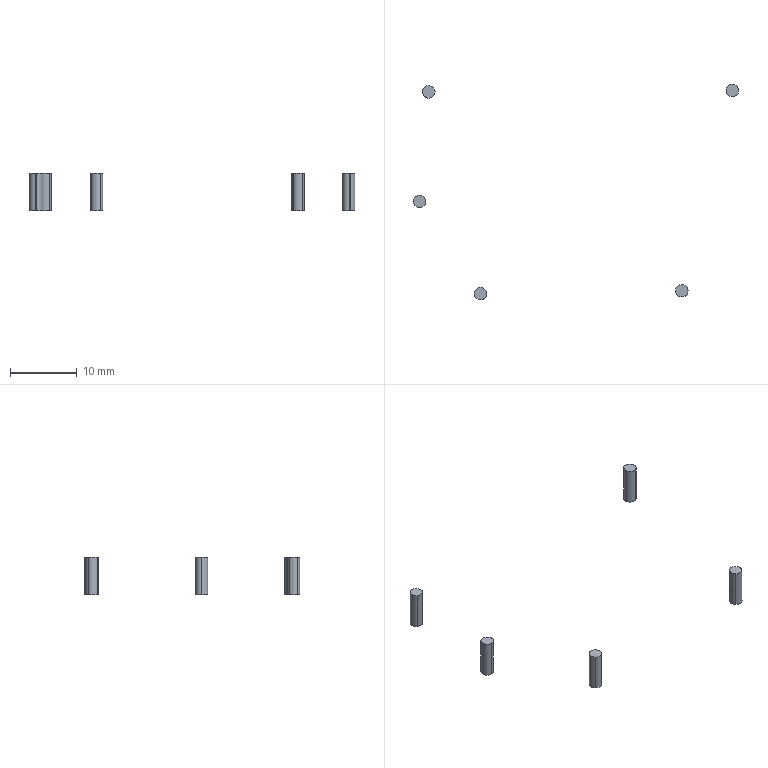Part | STEP file | TQ-DD-1105-THCoil21010_デフォルト | 5 solids | 55 faces | box 48.573 x 32.204 x 5.639 mm | volume 77.064 mm3 | plane 30 | cylinder 25 | commonest cylinder face diameters 1.84 x25